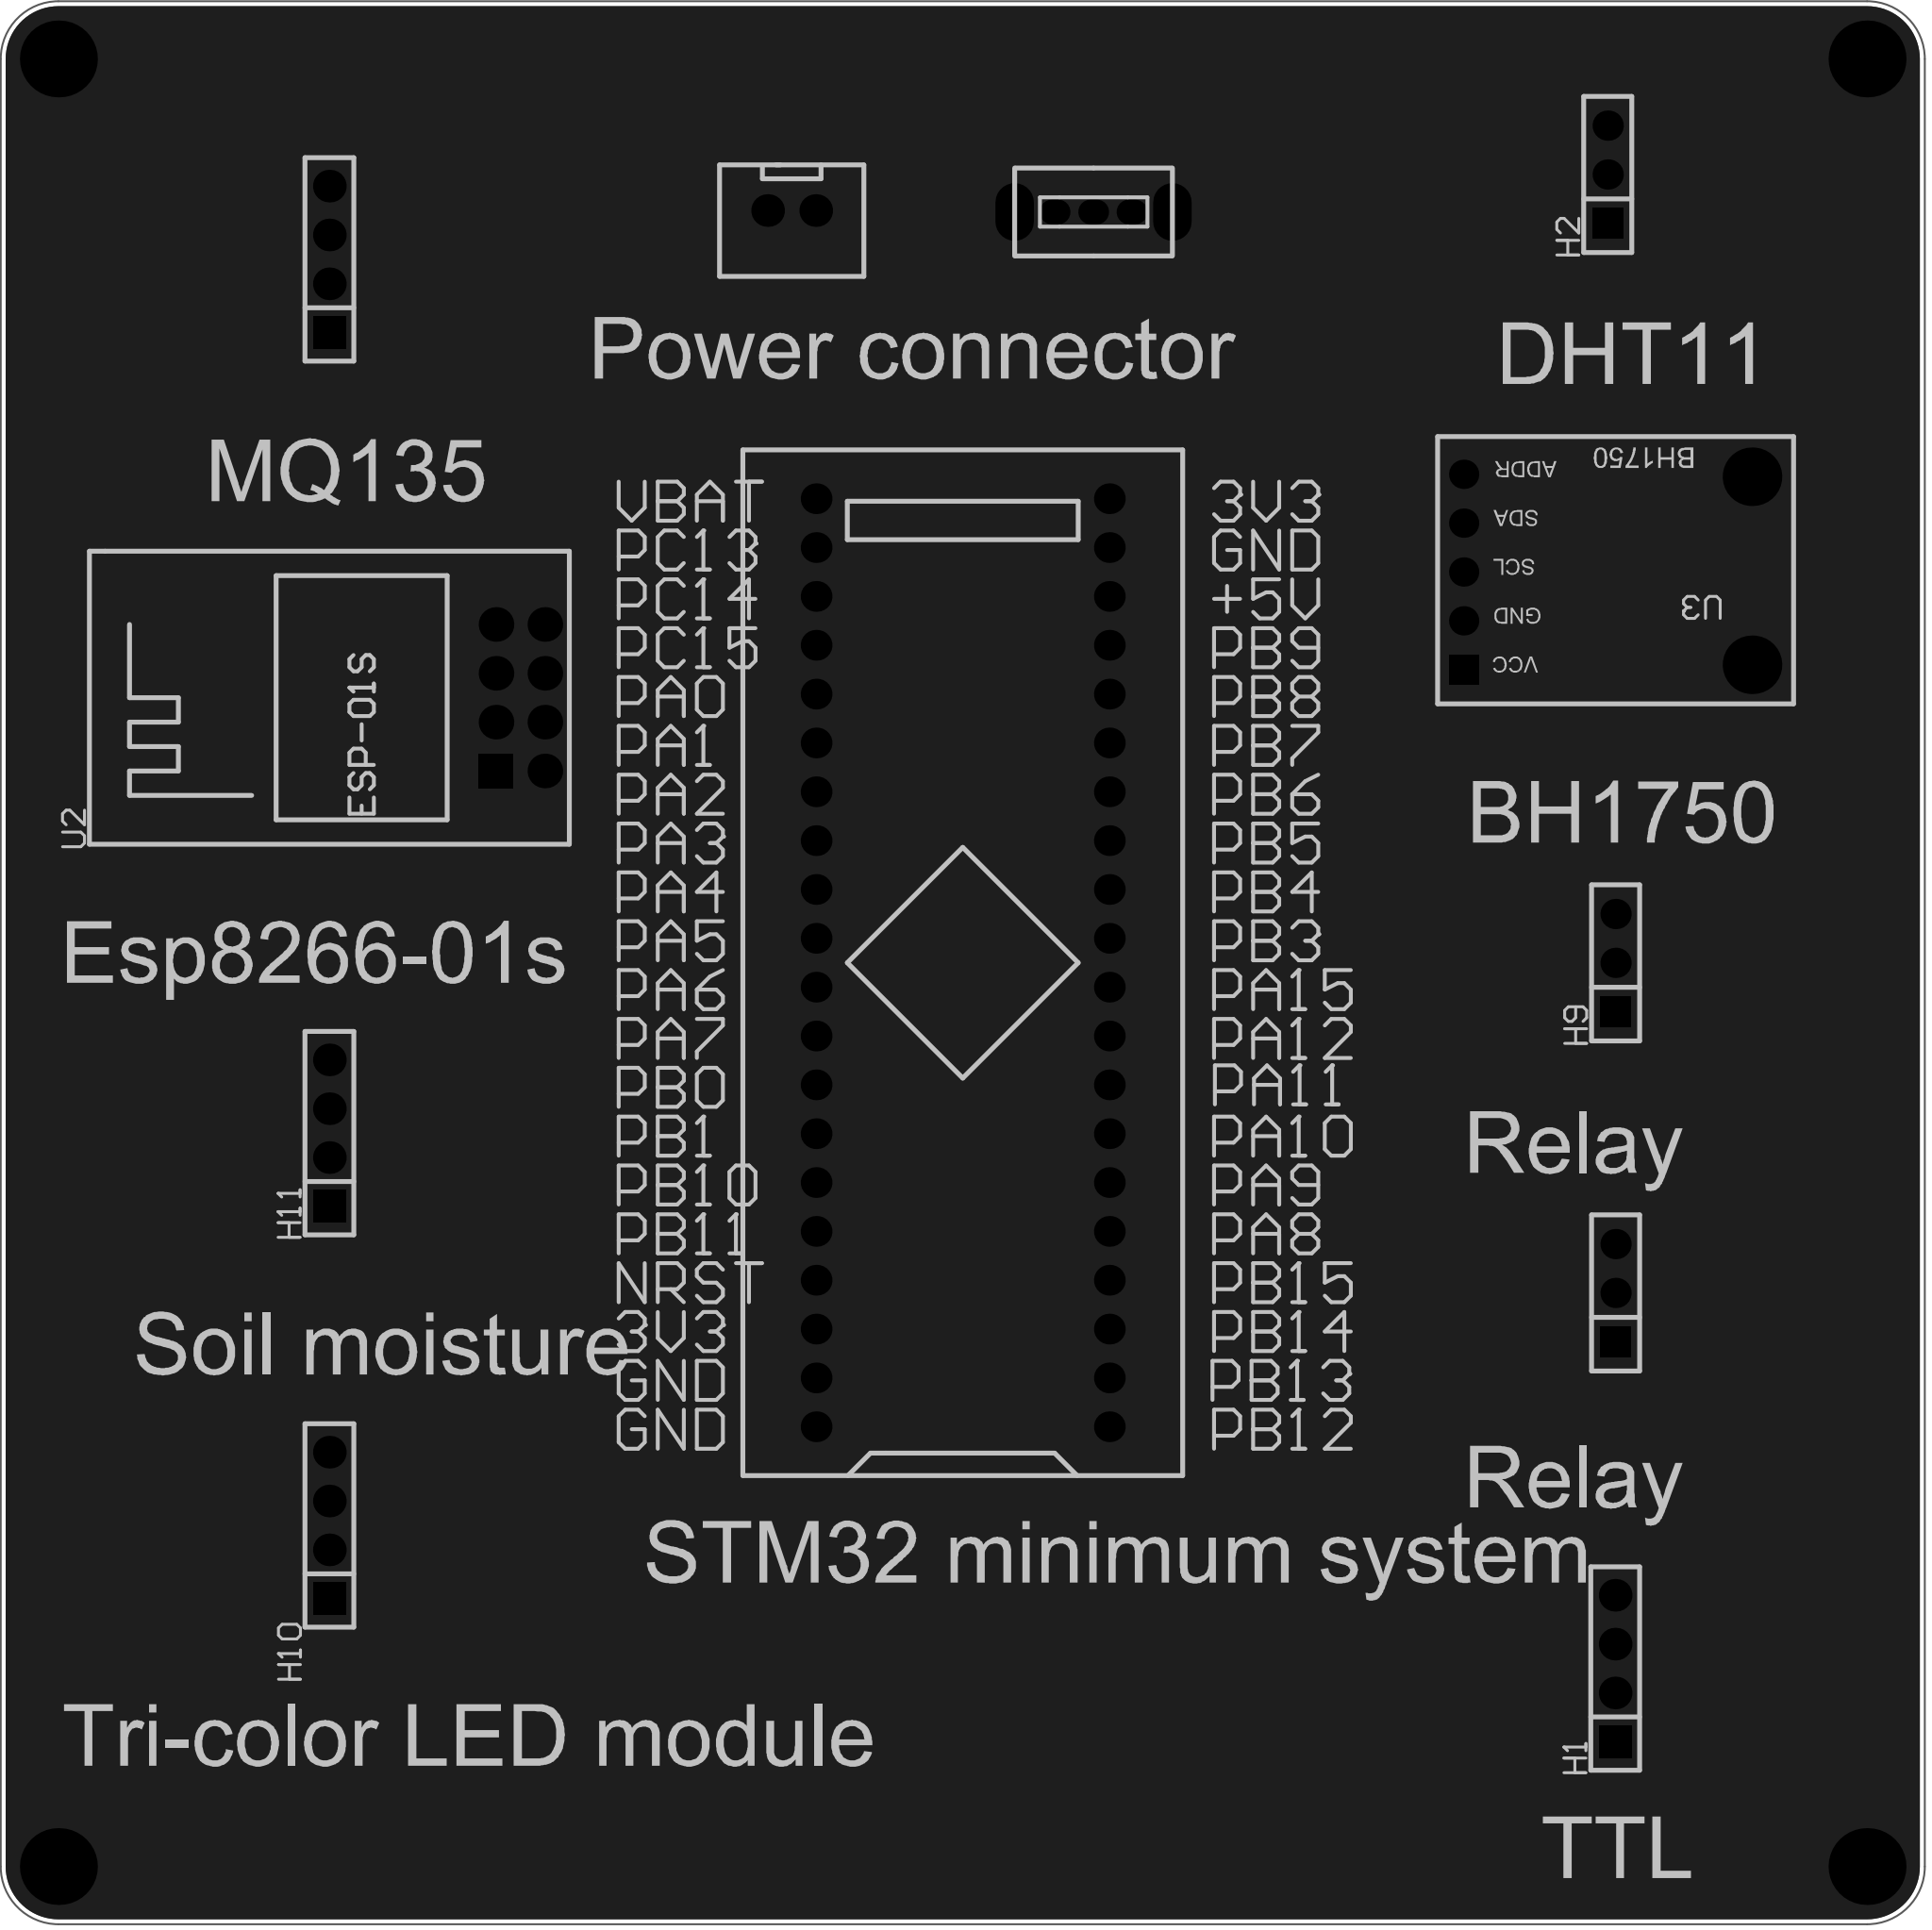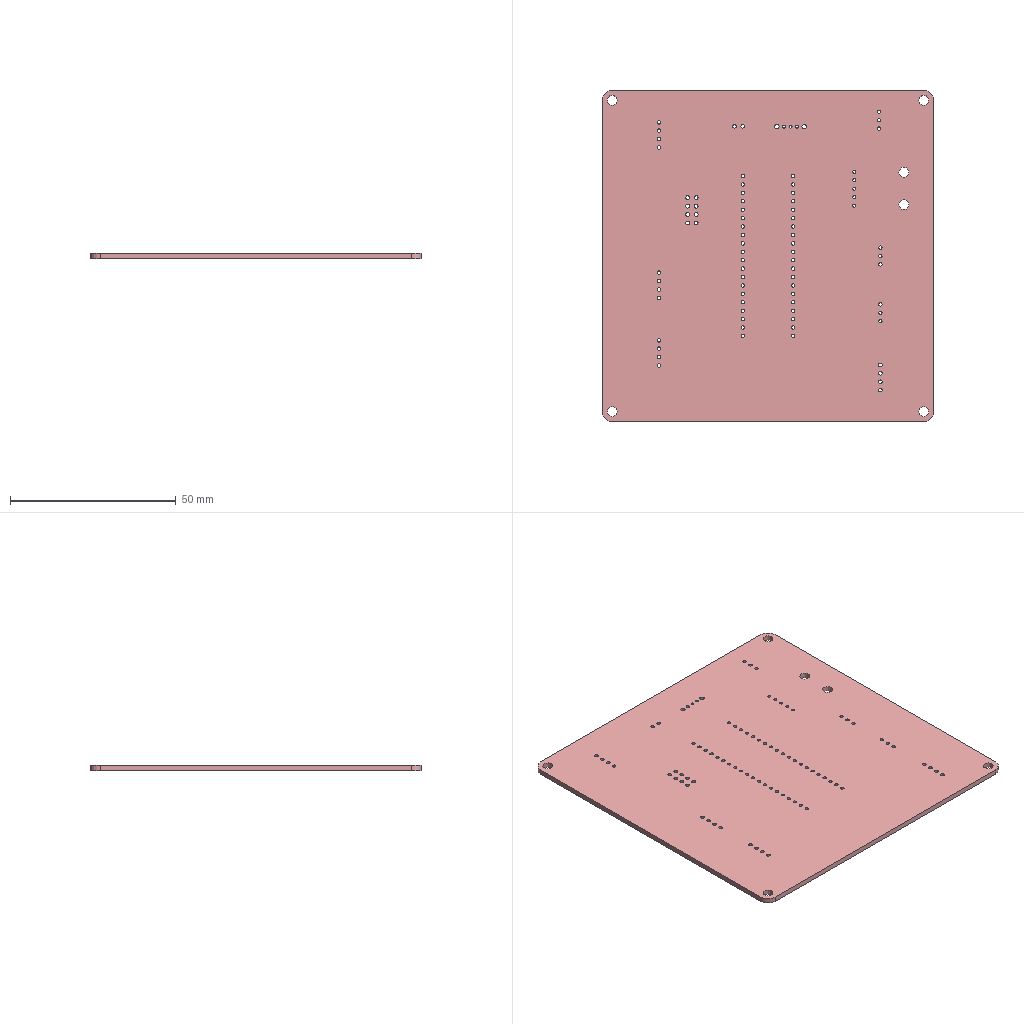Circuit board layout | Altium Designer | box 100 x 100 x 1.6 mm
Layer stack:
# Altium Designer layer stack of  (unit mm; dielectric type: 0 none, 1 core, 2 prepreg, 3 surface material)
index,name,kind,layer,copper_thickness_mm,dielectric_type,dielectric_thickness_mm,dielectric_material,dielectric_constant
0,Top Paste Mask Layer,other,,,,,,
1,Top Silkscreen Layer,other,,,,,,
2,Top Solder Mask Layer,dielectric,,,3,0.01,,3.3
3,Top Layer,copper,Top Layer,0.035,,,,
4,Dielectric1,dielectric,,,3,1.51,FR4,4.5
5,Bottom Layer,copper,Bottom Layer,0.035,,,,
6,Bottom Solder Mask Layer,dielectric,,,3,0.01,,3.3
7,Bottom Silkscreen Layer,other,,,,,,
8,Bottom Paste Mask Layer,other,,,,,,
# drill layer pairs: low layer,high layer
drill_pair,Top Layer,Bottom Layer
Part placement:
Designator,Comment,Layer,Footprint,Center-X(mm),Center-Y(mm),Rotation
U1,STM32F103C8T6-Card,TopLayer,CONN-TH_L53.3-W22.9_STM32F103C8T6-CARD,141.351,130.937,90
CN4,XH2.54*2P_straight,TopLayer,CONN-TH_2P-P2.50-XH2.54-2P,132.461,170.053,0
SW5,,TopLayer,拨动开关,148.148,169.978,180
H3,,TopLayer,HDR-TH_3P-P2.54-V-F,175.281,113.766,90
H4,,TopLayer,HDR-TH_4P-P2.54-V-F,108.433,167.513,90
H10,,TopLayer,HDR-TH_4P-P2.54-V-F,108.433,101.675,90
U3,,TopLayer,BH1750光照传感器,174.879,151.257,180
H9,,TopLayer,HDR-TH_3P-P2.54-V-F,175.281,130.931,90
H11,,TopLayer,HDR-TH_4P-P2.54-V-F,108.433,122.076,90
U2,ESP-01S,TopLayer,WIFIM-TH_ESP-01S,118.364,144.719,90
H1,,TopLayer,HDR-TH_4P-P2.54-V-F,175.26,94.234,90
H2,,TopLayer,HDR-TH_3P-P2.54-V-F,174.873,171.929,90
Pad and via stacks:
# Altium Designer via and pad stacks of  (unit mm). Each distinct definition once, with the count of objects using it.
# via: kind,start_layer,end_layer,hole_mm,diameter_mm,mode(0 simple;1 top-mid-bottom;2 full stack),diameter_per_layer,count,example_net
# pad: kind,layer,hole_mm,hole_type(0 round;1 square;2 slot),plating,top_size,top_shape(1 round;2 rect;3 octagon;9 rounded rect),mid_size,bottom_size,mode,footprint,size_per_layer,count,example
pad,Multi-Layer,3,0,plated,4x4,1,4x4,4x4,0,,,4,1
pad,Multi-Layer,1,0,plated,1.6x1.6,1,1.6x1.6,1.6x1.6,0,CONN-TH_L53.3-W22.9_STM32F103C8T6-CARD,,40,U1.1
pad,Multi-Layer,1.05,0,plated,1.7x1.7,1,1.7x1.7,1.7x1.7,0,CONN-TH_2P-P2.50-XH2.54-2P,,2,CN4.2
pad,Multi-Layer,0.8992,0,plated,1.6x1.3,1,1.6x1.3,1.6x1.3,0,\u00B2\u00A6\u00B6\u00AF\u00BF\u00AA\u00B9\u00D8,,3,SW5.1
pad,Multi-Layer,1.3,0,plated,3x1.999,1,3x1.999,3x1.999,0,\u00B2\u00A6\u00B6\u00AF\u00BF\u00AA\u00B9\u00D8,,2,SW5.4
pad,Multi-Layer,1.02,0,plated,1.575x1.575,1,1.575x1.575,1.575x1.575,0,HDR-TH_3P-P2.54-V-F,,6,H3.3
pad,Multi-Layer,1.02,0,plated,1.575x1.575,2,1.575x1.575,1.575x1.575,0,HDR-TH_3P-P2.54-V-F,,3,H3.1
pad,Multi-Layer,1.1,0,plated,1.7x1.7,2,1.7x1.7,1.7x1.7,0,HDR-TH_4P-P2.54-V-F,,4,H4.1
pad,Multi-Layer,1.1,0,plated,1.7x1.7,1,1.7x1.7,1.7x1.7,0,HDR-TH_4P-P2.54-V-F,,12,H4.2
pad,Multi-Layer,3.048,0,unplated,3.048x3.048,1,3.048x3.048,3.048x3.048,0,BH1750\u00B9\u00E2\u00D5\u00D5\u00B4\u00AB\u00B8\u00D0\u00C6\u00F7,,2,U3.
pad,Multi-Layer,0.9144,0,plated,1.524x1.524,2,1.524x1.524,1.524x1.524,0,BH1750\u00B9\u00E2\u00D5\u00D5\u00B4\u00AB\u00B8\u00D0\u00C6\u00F7,,1,U3.1
pad,Multi-Layer,0.9144,0,plated,1.524x1.524,1,1.524x1.524,1.524x1.524,0,BH1750\u00B9\u00E2\u00D5\u00D5\u00B4\u00AB\u00B8\u00D0\u00C6\u00F7,,4,U3.4
pad,Multi-Layer,1.2,0,plated,1.8x1.8,2,1.8x1.8,1.8x1.8,0,WIFIM-TH_ESP-01S,,1,U2.1
pad,Multi-Layer,1.2,0,plated,1.8x1.8,1,1.8x1.8,1.8x1.8,0,WIFIM-TH_ESP-01S,,7,U2.2
Copper pours:
name,layer,net,type(0 solid;1 hatched;2 none)
Bottom Layer-GND,Bottom Layer,GND,0
Top Layer-GND,Top Layer,GND,0
Design rules, without the lines most boards share:
# Altium Designer design rules of  (exported by Altium Designer, unit mm)
# columns: name | kind | enabled | priority | scope1 | scope2 | descriptor | typed fields (field=value)
Copper_copperRegion_copperThickness1oz | 0 | disabled | 4 | All | All | Clearance Constraint (Gap=5.984mil) (Disabled)(All),(All) | gap=0.152
Copper_copperRegion_copperThickness1oz_1 | 63 | disabled | 4 | All | All | Board Clearance Constraint (Gap=0mil) (Disabled)(All) |
Copper_copperRegion_Copper_copperRegion | 0 | disabled | 5 | All | All | Clearance Constraint (Gap=5.984mil) (Disabled)(All),(All) | gap=0.152
Copper_copperRegion_Copper_copperRegion_1 | 63 | disabled | 5 | All | All | Board Clearance Constraint (Gap=0mil) (Disabled)(All) |
copperThickness1oz | 0 | enabled | 6 | All | All | Clearance Constraint (Gap=5.984mil) (All),(All) | gap=0.152
copperThickness1oz_1 | 63 | enabled | 6 | All | All | Board Clearance Constraint (Gap=0mil) (All) |
copperRegion_copperThickness1oz | 20 | disabled | 1 | All | All | Polygon Connect Rule(Relief Connect )(Conductor Width=10mil) (Relief Angle=90 Angle) (Entries=4) (Air Gap Width=10mil) (Disabled)(All),(All) | connect_style(0=relief,1=direct,2=none)=0 relief_conductor_width=0.254 relief_entries=4
copperRegion_Copper_copperRegion | 20 | disabled | 2 | All | All | Polygon Connect Rule(Relief Connect )(Conductor Width=10mil) (Relief Angle=90 Angle) (Entries=4) (Air Gap Width=10mil) (Disabled)(All),(All) | connect_style(0=relief,1=direct,2=none)=0 relief_conductor_width=0.254 relief_entries=4
copperRegion | 20 | enabled | 3 | All | All | Polygon Connect Rule(Relief Connect )(Conductor Width=10mil) (Relief Angle=90 Angle) (Entries=4) (Air Gap Width=10mil) (All),(All) | connect_style(0=relief,1=direct,2=none)=0 relief_conductor_width=0.254 relief_entries=4